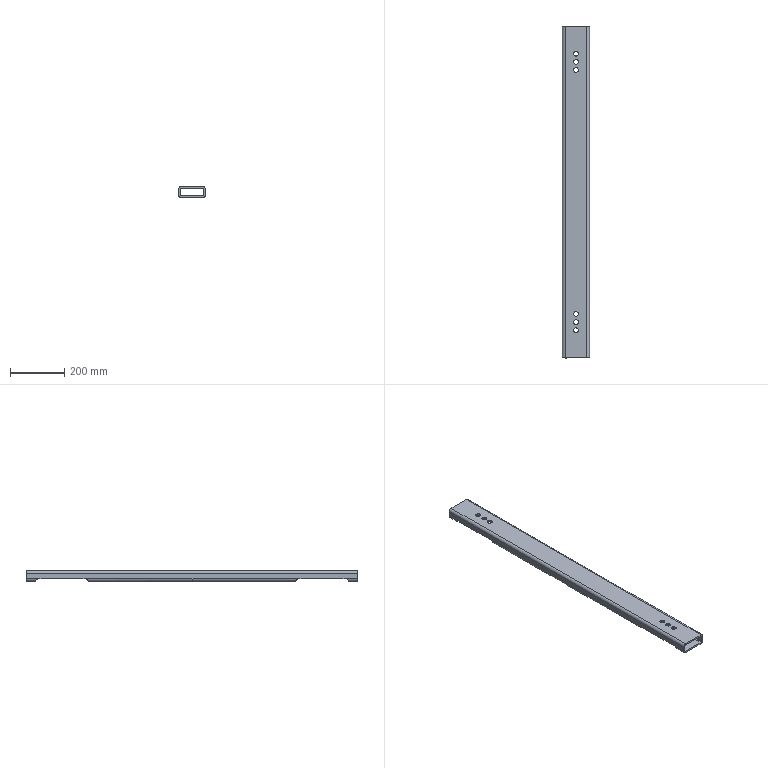Part | NX | features BREP 1 | 1 solid | 86 faces | box 100.003 x 1225 x 40 mm | volume 1550034 mm3 | cylinder 46 | plane 40 | commonest cylinder face diameters 8 x20 20 x14 17 x12